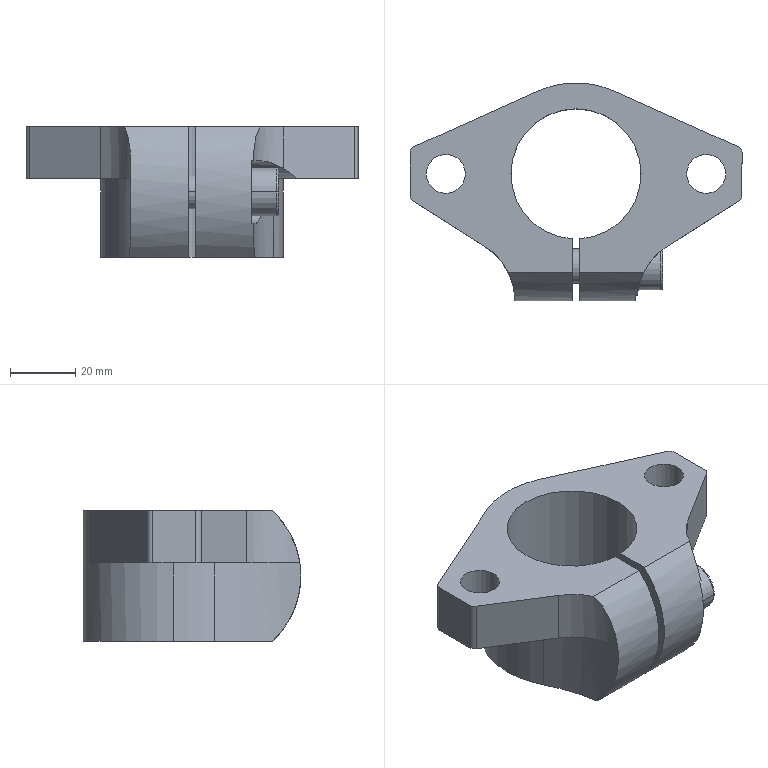Part | SolidWorks | features BaseBody 1 | 1 solid | 50 faces | box 102 x 67 x 40 mm | volume 87139 mm3 | cylinder 25 | plane 23 | spline 2 | commonest cylinder face diameters 4.02 x4 12 x4 40 x3 56 x3 10.5 x2 14.7 x2